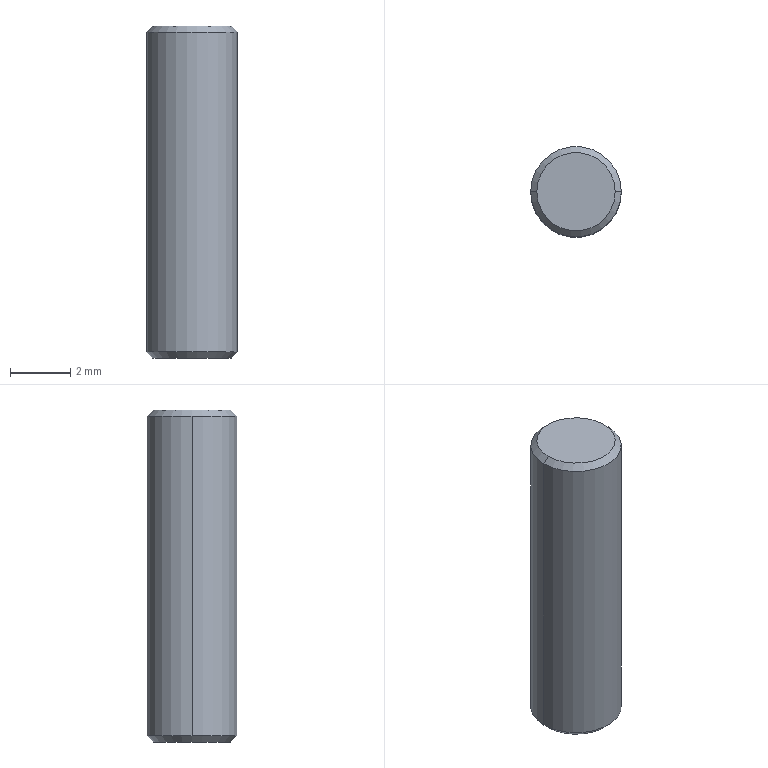Part | SolidWorks | features Chamfer 1, Extrusion 1 | 1 solid | 8 faces | box 3 x 3 x 11 mm | volume 77.394 mm3 | cone 4 | cylinder 2 | plane 2 | commonest cylinder face diameters 3 x2
STEP:
#1=CARTESIAN_POINT('',(-1.3,8.569,-11.));
#2=VERTEX_POINT('',#1);
#3=CARTESIAN_POINT('',(1.3,8.569,-11.));
#4=VERTEX_POINT('',#3);
#5=CARTESIAN_POINT('',(0.,8.569,-11.));
#6=DIRECTION('',(0.,0.,-1.));
#7=DIRECTION('',(1.,0.,0.));
#8=AXIS2_PLACEMENT_3D('',#5,#6,#7);
#9=CIRCLE('',#8,1.3);
#10=EDGE_CURVE('',#2,#4,#9,.T.);
#11=ORIENTED_EDGE('',*,*,#10,.F.);
#12=CARTESIAN_POINT('',(-1.5,8.569,-10.8));
#13=VERTEX_POINT('',#12);
#14=CARTESIAN_POINT('',(-1.5,8.569,-10.8));
#15=DIRECTION('',(-0.7071,0.,0.7071));
#16=VECTOR('',#15,1000.);
#17=LINE('',#14,#16);
#18=EDGE_CURVE('',#2,#13,#17,.T.);
#19=ORIENTED_EDGE('',*,*,#18,.T.);
#20=CARTESIAN_POINT('',(1.5,8.569,-10.8));
#21=VERTEX_POINT('',#20);
#22=CARTESIAN_POINT('',(0.,8.569,-10.8));
#23=DIRECTION('',(0.,0.,1.));
#24=DIRECTION('',(1.,0.,0.));
#25=AXIS2_PLACEMENT_3D('',#22,#23,#24);
#26=CIRCLE('',#25,1.5);
#27=EDGE_CURVE('',#21,#13,#26,.T.);
#28=ORIENTED_EDGE('',*,*,#27,.F.);
#29=CARTESIAN_POINT('',(1.5,8.569,-10.8));
#30=DIRECTION('',(0.7071,0.,0.7071));
#31=VECTOR('',#30,1000.);
#32=LINE('',#29,#31);
#33=EDGE_CURVE('',#4,#21,#32,.T.);
#34=ORIENTED_EDGE('',*,*,#33,.F.);
#35=EDGE_LOOP('',(#11,#19,#28,#34));
#36=FACE_OUTER_BOUND('',#35,.T.);
#37=CARTESIAN_POINT('',(0.,8.569,-10.8));
#38=DIRECTION('',(0.,0.,1.));
#39=DIRECTION('',(1.,0.,0.));
#40=AXIS2_PLACEMENT_3D('',#37,#38,#39);
#41=CONICAL_SURFACE('',#40,1.5,0.7854);
#42=ADVANCED_FACE('',(#36),#41,.T.);
#43=CARTESIAN_POINT('',(1.3,8.569,0.));
#44=VERTEX_POINT('',#43);
#45=CARTESIAN_POINT('',(-1.3,8.569,0.));
#46=VERTEX_POINT('',#45);
#47=CARTESIAN_POINT('',(0.,8.569,0.));
#48=DIRECTION('',(0.,0.,1.));
#49=DIRECTION('',(1.,0.,0.));
#50=AXIS2_PLACEMENT_3D('',#47,#48,#49);
#51=CIRCLE('',#50,1.3);
#52=EDGE_CURVE('',#44,#46,#51,.T.);
#53=ORIENTED_EDGE('',*,*,#52,.F.);
#54=CARTESIAN_POINT('',(1.5,8.569,-0.2));
#55=VERTEX_POINT('',#54);
#56=CARTESIAN_POINT('',(1.3,8.569,0.));
#57=DIRECTION('',(0.7071,0.,-0.7071));
#58=VECTOR('',#57,1000.);
#59=LINE('',#56,#58);
#60=EDGE_CURVE('',#44,#55,#59,.T.);
#61=ORIENTED_EDGE('',*,*,#60,.T.);
#62=CARTESIAN_POINT('',(-1.5,8.569,-0.2));
#63=VERTEX_POINT('',#62);
#64=CARTESIAN_POINT('',(0.,8.569,-0.2));
#65=DIRECTION('',(0.,0.,-1.));
#66=DIRECTION('',(1.,0.,0.));
#67=AXIS2_PLACEMENT_3D('',#64,#65,#66);
#68=CIRCLE('',#67,1.5);
#69=EDGE_CURVE('',#63,#55,#68,.T.);
#70=ORIENTED_EDGE('',*,*,#69,.F.);
#71=CARTESIAN_POINT('',(-1.3,8.569,0.));
#72=DIRECTION('',(-0.7071,0.,-0.7071));
#73=VECTOR('',#72,1000.);
#74=LINE('',#71,#73);
#75=EDGE_CURVE('',#46,#63,#74,.T.);
#76=ORIENTED_EDGE('',*,*,#75,.F.);
#77=EDGE_LOOP('',(#53,#61,#70,#76));
#78=FACE_OUTER_BOUND('',#77,.T.);
#79=CARTESIAN_POINT('',(0.,8.569,0.));
#80=DIRECTION('',(0.,0.,-1.));
#81=DIRECTION('',(-1.,0.,0.));
#82=AXIS2_PLACEMENT_3D('',#79,#80,#81);
#83=CONICAL_SURFACE('',#82,1.3,0.7854);
#84=ADVANCED_FACE('',(#78),#83,.T.);
#85=ORIENTED_EDGE('',*,*,#27,.T.);
#86=CARTESIAN_POINT('',(-1.5,8.569,-11.));
#87=DIRECTION('',(0.,0.,1.));
#88=VECTOR('',#87,1000.);
#89=LINE('',#86,#88);
#90=EDGE_CURVE('',#13,#63,#89,.T.);
#91=ORIENTED_EDGE('',*,*,#90,.T.);
#92=ORIENTED_EDGE('',*,*,#69,.T.);
#93=CARTESIAN_POINT('',(1.5,8.569,-11.));
#94=DIRECTION('',(0.,0.,1.));
#95=VECTOR('',#94,1000.);
#96=LINE('',#93,#95);
#97=EDGE_CURVE('',#21,#55,#96,.T.);
#98=ORIENTED_EDGE('',*,*,#97,.F.);
#99=EDGE_LOOP('',(#85,#91,#92,#98));
#100=FACE_OUTER_BOUND('',#99,.T.);
#101=CARTESIAN_POINT('',(0.,8.569,-11.));
#102=DIRECTION('',(0.,0.,1.));
#103=DIRECTION('',(1.,0.,0.));
#104=AXIS2_PLACEMENT_3D('',#101,#102,#103);
#105=CYLINDRICAL_SURFACE('',#104,1.5);
#106=ADVANCED_FACE('',(#100),#105,.T.);
#107=ORIENTED_EDGE('',*,*,#90,.F.);
#108=CARTESIAN_POINT('',(0.,8.569,-10.8));
#109=DIRECTION('',(0.,0.,1.));
#110=DIRECTION('',(1.,0.,0.));
#111=AXIS2_PLACEMENT_3D('',#108,#109,#110);
#112=CIRCLE('',#111,1.5);
#113=EDGE_CURVE('',#13,#21,#112,.T.);
#114=ORIENTED_EDGE('',*,*,#113,.T.);
#115=ORIENTED_EDGE('',*,*,#97,.T.);
#116=CARTESIAN_POINT('',(0.,8.569,-0.2));
#117=DIRECTION('',(0.,0.,-1.));
#118=DIRECTION('',(1.,0.,0.));
#119=AXIS2_PLACEMENT_3D('',#116,#117,#118);
#120=CIRCLE('',#119,1.5);
#121=EDGE_CURVE('',#55,#63,#120,.T.);
#122=ORIENTED_EDGE('',*,*,#121,.T.);
#123=EDGE_LOOP('',(#107,#114,#115,#122));
#124=FACE_OUTER_BOUND('',#123,.T.);
#125=CARTESIAN_POINT('',(0.,8.569,-11.));
#126=DIRECTION('',(0.,0.,1.));
#127=DIRECTION('',(1.,0.,0.));
#128=AXIS2_PLACEMENT_3D('',#125,#126,#127);
#129=CYLINDRICAL_SURFACE('',#128,1.5);
#130=ADVANCED_FACE('',(#124),#129,.T.);
#131=CARTESIAN_POINT('',(0.,8.569,-11.));
#132=DIRECTION('',(0.,0.,-1.));
#133=DIRECTION('',(1.,0.,0.));
#134=AXIS2_PLACEMENT_3D('',#131,#132,#133);
#135=CIRCLE('',#134,1.3);
#136=EDGE_CURVE('',#4,#2,#135,.T.);
#137=ORIENTED_EDGE('',*,*,#136,.T.);
#138=ORIENTED_EDGE('',*,*,#10,.T.);
#139=EDGE_LOOP('',(#137,#138));
#140=FACE_OUTER_BOUND('',#139,.T.);
#141=CARTESIAN_POINT('',(0.,8.569,-11.));
#142=DIRECTION('',(0.,0.,1.));
#143=DIRECTION('',(1.,0.,0.));
#144=AXIS2_PLACEMENT_3D('',#141,#142,#143);
#145=PLANE('',#144);
#146=ADVANCED_FACE('',(#140),#145,.F.);
#147=CARTESIAN_POINT('',(0.,8.569,0.));
#148=DIRECTION('',(0.,0.,1.));
#149=DIRECTION('',(1.,0.,0.));
#150=AXIS2_PLACEMENT_3D('',#147,#148,#149);
#151=CIRCLE('',#150,1.3);
#152=EDGE_CURVE('',#46,#44,#151,.T.);
#153=ORIENTED_EDGE('',*,*,#152,.T.);
#154=ORIENTED_EDGE('',*,*,#52,.T.);
#155=EDGE_LOOP('',(#153,#154));
#156=FACE_OUTER_BOUND('',#155,.T.);
#157=CARTESIAN_POINT('',(0.,8.569,0.));
#158=DIRECTION('',(0.,0.,1.));
#159=DIRECTION('',(1.,0.,0.));
#160=AXIS2_PLACEMENT_3D('',#157,#158,#159);
#161=PLANE('',#160);
#162=ADVANCED_FACE('',(#156),#161,.T.);
#163=ORIENTED_EDGE('',*,*,#60,.F.);
#164=ORIENTED_EDGE('',*,*,#152,.F.);
#165=ORIENTED_EDGE('',*,*,#75,.T.);
#166=ORIENTED_EDGE('',*,*,#121,.F.);
#167=EDGE_LOOP('',(#163,#164,#165,#166));
#168=FACE_OUTER_BOUND('',#167,.T.);
#169=CARTESIAN_POINT('',(0.,8.569,0.));
#170=DIRECTION('',(0.,0.,-1.));
#171=DIRECTION('',(-1.,0.,0.));
#172=AXIS2_PLACEMENT_3D('',#169,#170,#171);
#173=CONICAL_SURFACE('',#172,1.3,0.7854);
#174=ADVANCED_FACE('',(#168),#173,.T.);
#175=ORIENTED_EDGE('',*,*,#18,.F.);
#176=ORIENTED_EDGE('',*,*,#136,.F.);
#177=ORIENTED_EDGE('',*,*,#33,.T.);
#178=ORIENTED_EDGE('',*,*,#113,.F.);
#179=EDGE_LOOP('',(#175,#176,#177,#178));
#180=FACE_OUTER_BOUND('',#179,.T.);
#181=CARTESIAN_POINT('',(0.,8.569,-10.8));
#182=DIRECTION('',(0.,0.,1.));
#183=DIRECTION('',(1.,0.,0.));
#184=AXIS2_PLACEMENT_3D('',#181,#182,#183);
#185=CONICAL_SURFACE('',#184,1.5,0.7854);
#186=ADVANCED_FACE('',(#180),#185,.T.);
#187=CLOSED_SHELL('',(#42,#84,#106,#130,#146,#162,#174,#186));
#188=MANIFOLD_SOLID_BREP('',#187);
#189=CARTESIAN_POINT('',(0.,0.,0.));
#190=DIRECTION('',(0.,0.,1.));
#191=DIRECTION('',(1.,0.,0.));
#192=AXIS2_PLACEMENT_3D('',#189,#190,#191);
#193=(LENGTH_UNIT()NAMED_UNIT(*)SI_UNIT(.MILLI.,.METRE.));
#194=UNCERTAINTY_MEASURE_WITH_UNIT(LENGTH_MEASURE(0.00001),#193,'','');
#195=(NAMED_UNIT(*)PLANE_ANGLE_UNIT()SI_UNIT($,.RADIAN.));
#196=(NAMED_UNIT(*)SI_UNIT($,.STERADIAN.)SOLID_ANGLE_UNIT());
#197=(GEOMETRIC_REPRESENTATION_CONTEXT(3)GLOBAL_UNCERTAINTY_ASSIGNED_CONTEXT((#194))GLOBAL_UNIT_ASSIGNED_CONTEXT((#193,#195,#196))REPRESENTATION_CONTEXT('',''));
#198=ADVANCED_BREP_SHAPE_REPRESENTATION('',(#188,#192),#197);